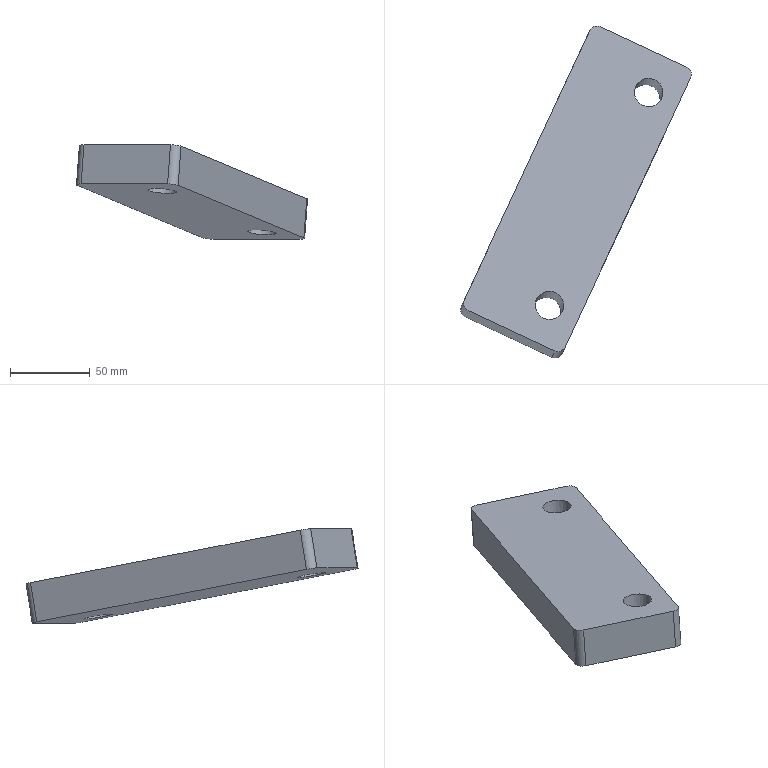Part | NX | features MAIN_BODY 2 | 1 solid | 12 faces | box 145.264 x 208.749 x 59.35 mm | volume 336740 mm3 | plane 6 | cylinder 6 | commonest cylinder face diameters 10 x4 18 x2
STEP:
#1=CARTESIAN_POINT('',(608.13,416.814,55.362));
#2=VERTEX_POINT('',#1);
#3=CARTESIAN_POINT('',(662.509,391.456,55.362));
#4=VERTEX_POINT('',#3);
#5=CARTESIAN_POINT('',(603.599,418.927,55.362));
#6=DIRECTION('',(0.9063,-0.4226,0.000000004));
#7=VECTOR('',#6,1000.);
#8=LINE('',#5,#7);
#9=EDGE_CURVE('',#2,#4,#8,.T.);
#10=ORIENTED_EDGE('',*,*,#9,.T.);
#11=CARTESIAN_POINT('',(664.343,395.391,79.982));
#12=VERTEX_POINT('',#11);
#13=CARTESIAN_POINT('',(664.343,395.391,79.982));
#14=DIRECTION('',(-0.07339,-0.1574,-0.9848));
#15=VECTOR('',#14,1000.);
#16=LINE('',#13,#15);
#17=EDGE_CURVE('',#12,#4,#16,.T.);
#18=ORIENTED_EDGE('',*,*,#17,.F.);
#19=CARTESIAN_POINT('',(609.965,420.748,79.982));
#20=VERTEX_POINT('',#19);
#21=CARTESIAN_POINT('',(605.433,422.861,79.982));
#22=DIRECTION('',(0.9063,-0.4226,0.000000004));
#23=VECTOR('',#22,1000.);
#24=LINE('',#21,#23);
#25=EDGE_CURVE('',#20,#12,#24,.T.);
#26=ORIENTED_EDGE('',*,*,#25,.F.);
#27=CARTESIAN_POINT('',(609.965,420.748,79.982));
#28=DIRECTION('',(-0.07339,-0.1574,-0.9848));
#29=VECTOR('',#28,1000.);
#30=LINE('',#27,#29);
#31=EDGE_CURVE('',#2,#20,#30,.F.);
#32=ORIENTED_EDGE('',*,*,#31,.F.);
#33=EDGE_LOOP('',(#10,#18,#26,#32));
#34=FACE_BOUND('',#33,.T.);
#35=CARTESIAN_POINT('',(605.433,422.861,79.982));
#36=DIRECTION('',(-0.4162,-0.8925,0.1736));
#37=DIRECTION('',(-0.9063,0.4226,-0.000000004));
#38=AXIS2_PLACEMENT_3D('',#35,#36,#37);
#39=PLANE('',#38);
#40=ADVANCED_FACE('',(#34),#39,.T.);
#41=CARTESIAN_POINT('',(670.956,397.741,79.114));
#42=VERTEX_POINT('',#41);
#43=CARTESIAN_POINT('',(750.033,567.323,46.121));
#44=VERTEX_POINT('',#43);
#45=CARTESIAN_POINT('',(668.875,393.278,79.982));
#46=DIRECTION('',(0.4162,0.8925,-0.1736));
#47=VECTOR('',#46,1000.);
#48=LINE('',#45,#47);
#49=EDGE_CURVE('',#42,#44,#48,.T.);
#50=ORIENTED_EDGE('',*,*,#49,.F.);
#51=CARTESIAN_POINT('',(669.121,393.806,54.494));
#52=VERTEX_POINT('',#51);
#53=CARTESIAN_POINT('',(670.956,397.741,79.114));
#54=DIRECTION('',(-0.07339,-0.1574,-0.9848));
#55=VECTOR('',#54,1000.);
#56=LINE('',#53,#55);
#57=EDGE_CURVE('',#52,#42,#56,.F.);
#58=ORIENTED_EDGE('',*,*,#57,.F.);
#59=CARTESIAN_POINT('',(748.199,563.388,21.501));
#60=VERTEX_POINT('',#59);
#61=CARTESIAN_POINT('',(667.04,389.343,55.362));
#62=DIRECTION('',(0.4162,0.8925,-0.1736));
#63=VECTOR('',#62,1000.);
#64=LINE('',#61,#63);
#65=EDGE_CURVE('',#52,#60,#64,.T.);
#66=ORIENTED_EDGE('',*,*,#65,.T.);
#67=CARTESIAN_POINT('',(750.033,567.323,46.121));
#68=DIRECTION('',(-0.07339,-0.1574,-0.9848));
#69=VECTOR('',#68,1000.);
#70=LINE('',#67,#69);
#71=EDGE_CURVE('',#44,#60,#70,.T.);
#72=ORIENTED_EDGE('',*,*,#71,.F.);
#73=EDGE_LOOP('',(#50,#58,#66,#72));
#74=FACE_BOUND('',#73,.T.);
#75=CARTESIAN_POINT('',(668.875,393.278,79.982));
#76=DIRECTION('',(0.9063,-0.4226,0.000000004));
#77=DIRECTION('',(-0.4162,-0.8925,0.1736));
#78=AXIS2_PLACEMENT_3D('',#75,#76,#77);
#79=PLANE('',#78);
#80=ADVANCED_FACE('',(#74),#79,.T.);
#81=CARTESIAN_POINT('',(747.583,573.899,45.252));
#82=VERTEX_POINT('',#81);
#83=CARTESIAN_POINT('',(693.204,599.256,45.252));
#84=VERTEX_POINT('',#83);
#85=CARTESIAN_POINT('',(752.114,571.786,45.252));
#86=DIRECTION('',(-0.9063,0.4226,-0.000000004));
#87=VECTOR('',#86,1000.);
#88=LINE('',#85,#87);
#89=EDGE_CURVE('',#82,#84,#88,.T.);
#90=ORIENTED_EDGE('',*,*,#89,.F.);
#91=CARTESIAN_POINT('',(745.748,569.964,20.632));
#92=VERTEX_POINT('',#91);
#93=CARTESIAN_POINT('',(747.583,573.899,45.252));
#94=DIRECTION('',(-0.07339,-0.1574,-0.9848));
#95=VECTOR('',#94,1000.);
#96=LINE('',#93,#95);
#97=EDGE_CURVE('',#92,#82,#96,.F.);
#98=ORIENTED_EDGE('',*,*,#97,.F.);
#99=CARTESIAN_POINT('',(691.37,595.321,20.632));
#100=VERTEX_POINT('',#99);
#101=CARTESIAN_POINT('',(750.28,567.851,20.632));
#102=DIRECTION('',(-0.9063,0.4226,-0.000000004));
#103=VECTOR('',#102,1000.);
#104=LINE('',#101,#103);
#105=EDGE_CURVE('',#92,#100,#104,.T.);
#106=ORIENTED_EDGE('',*,*,#105,.T.);
#107=CARTESIAN_POINT('',(693.204,599.256,45.252));
#108=DIRECTION('',(-0.07339,-0.1574,-0.9848));
#109=VECTOR('',#108,1000.);
#110=LINE('',#107,#109);
#111=EDGE_CURVE('',#84,#100,#110,.T.);
#112=ORIENTED_EDGE('',*,*,#111,.F.);
#113=EDGE_LOOP('',(#90,#98,#106,#112));
#114=FACE_BOUND('',#113,.T.);
#115=CARTESIAN_POINT('',(752.114,571.786,45.252));
#116=DIRECTION('',(0.4162,0.8925,-0.1736));
#117=DIRECTION('',(0.07339,0.1574,0.9848));
#118=AXIS2_PLACEMENT_3D('',#115,#116,#117);
#119=PLANE('',#118);
#120=ADVANCED_FACE('',(#114),#119,.T.);
#121=CARTESIAN_POINT('',(684.757,592.972,21.501));
#122=VERTEX_POINT('',#121);
#123=CARTESIAN_POINT('',(605.68,423.389,54.494));
#124=VERTEX_POINT('',#123);
#125=CARTESIAN_POINT('',(686.838,597.434,20.632));
#126=DIRECTION('',(-0.4162,-0.8925,0.1736));
#127=VECTOR('',#126,1000.);
#128=LINE('',#125,#127);
#129=EDGE_CURVE('',#122,#124,#128,.T.);
#130=ORIENTED_EDGE('',*,*,#129,.T.);
#131=CARTESIAN_POINT('',(607.514,427.324,79.114));
#132=VERTEX_POINT('',#131);
#133=CARTESIAN_POINT('',(607.514,427.324,79.114));
#134=DIRECTION('',(-0.07339,-0.1574,-0.9848));
#135=VECTOR('',#134,1000.);
#136=LINE('',#133,#135);
#137=EDGE_CURVE('',#132,#124,#136,.T.);
#138=ORIENTED_EDGE('',*,*,#137,.F.);
#139=CARTESIAN_POINT('',(686.592,596.906,46.121));
#140=VERTEX_POINT('',#139);
#141=CARTESIAN_POINT('',(688.673,601.369,45.252));
#142=DIRECTION('',(-0.4162,-0.8925,0.1736));
#143=VECTOR('',#142,1000.);
#144=LINE('',#141,#143);
#145=EDGE_CURVE('',#140,#132,#144,.T.);
#146=ORIENTED_EDGE('',*,*,#145,.F.);
#147=CARTESIAN_POINT('',(686.592,596.906,46.121));
#148=DIRECTION('',(-0.07339,-0.1574,-0.9848));
#149=VECTOR('',#148,1000.);
#150=LINE('',#147,#149);
#151=EDGE_CURVE('',#122,#140,#150,.F.);
#152=ORIENTED_EDGE('',*,*,#151,.F.);
#153=EDGE_LOOP('',(#130,#138,#146,#152));
#154=FACE_BOUND('',#153,.T.);
#155=CARTESIAN_POINT('',(688.673,601.369,45.252));
#156=DIRECTION('',(-0.9063,0.4226,-0.000000004));
#157=DIRECTION('',(0.07339,0.1574,0.9848));
#158=AXIS2_PLACEMENT_3D('',#155,#156,#157);
#159=PLANE('',#158);
#160=ADVANCED_FACE('',(#154),#159,.T.);
#161=CARTESIAN_POINT('',(727.329,565.957,48.031));
#162=VERTEX_POINT('',#161);
#163=CARTESIAN_POINT('',(723.583,557.925,49.594));
#164=DIRECTION('',(0.07339,0.1574,0.9848));
#165=DIRECTION('',(0.4162,0.8925,-0.1736));
#166=AXIS2_PLACEMENT_3D('',#163,#164,#165);
#167=CIRCLE('',#166,9.);
#168=EDGE_CURVE('',#162,#162,#167,.T.);
#169=ORIENTED_EDGE('',*,*,#168,.F.);
#170=EDGE_LOOP('',(#169));
#171=FACE_BOUND('',#170,.T.);
#172=CARTESIAN_POINT('',(664.899,432.077,74.078));
#173=VERTEX_POINT('',#172);
#174=CARTESIAN_POINT('',(661.154,424.044,75.641));
#175=DIRECTION('',(0.07339,0.1574,0.9848));
#176=DIRECTION('',(0.4162,0.8925,-0.1736));
#177=AXIS2_PLACEMENT_3D('',#174,#175,#176);
#178=CIRCLE('',#177,9.);
#179=EDGE_CURVE('',#173,#173,#178,.T.);
#180=ORIENTED_EDGE('',*,*,#179,.F.);
#181=EDGE_LOOP('',(#180));
#182=FACE_BOUND('',#181,.T.);
#183=ORIENTED_EDGE('',*,*,#145,.T.);
#184=CARTESIAN_POINT('',(612.046,425.211,79.114));
#185=DIRECTION('',(0.07339,0.1574,0.9848));
#186=DIRECTION('',(0.4162,0.8925,-0.1736));
#187=AXIS2_PLACEMENT_3D('',#184,#185,#186);
#188=CIRCLE('',#187,5.);
#189=EDGE_CURVE('',#20,#132,#188,.F.);
#190=ORIENTED_EDGE('',*,*,#189,.F.);
#191=ORIENTED_EDGE('',*,*,#25,.T.);
#192=CARTESIAN_POINT('',(666.424,399.854,79.114));
#193=DIRECTION('',(0.07339,0.1574,0.9848));
#194=DIRECTION('',(0.4162,0.8925,-0.1736));
#195=AXIS2_PLACEMENT_3D('',#192,#193,#194);
#196=CIRCLE('',#195,5.);
#197=EDGE_CURVE('',#42,#12,#196,.F.);
#198=ORIENTED_EDGE('',*,*,#197,.F.);
#199=ORIENTED_EDGE('',*,*,#49,.T.);
#200=CARTESIAN_POINT('',(745.502,569.436,46.121));
#201=DIRECTION('',(0.07339,0.1574,0.9848));
#202=DIRECTION('',(0.4162,0.8925,-0.1736));
#203=AXIS2_PLACEMENT_3D('',#200,#201,#202);
#204=CIRCLE('',#203,5.);
#205=EDGE_CURVE('',#82,#44,#204,.F.);
#206=ORIENTED_EDGE('',*,*,#205,.F.);
#207=ORIENTED_EDGE('',*,*,#89,.T.);
#208=CARTESIAN_POINT('',(691.123,594.793,46.121));
#209=DIRECTION('',(0.07339,0.1574,0.9848));
#210=DIRECTION('',(0.4162,0.8925,-0.1736));
#211=AXIS2_PLACEMENT_3D('',#208,#209,#210);
#212=CIRCLE('',#211,5.);
#213=EDGE_CURVE('',#140,#84,#212,.F.);
#214=ORIENTED_EDGE('',*,*,#213,.F.);
#215=EDGE_LOOP('',(#183,#190,#191,#198,#199,#206,#207,#214));
#216=FACE_BOUND('',#215,.T.);
#217=CARTESIAN_POINT('',(668.875,393.278,79.982));
#218=DIRECTION('',(-0.07339,-0.1574,-0.9848));
#219=DIRECTION('',(0.4162,0.8925,-0.1736));
#220=AXIS2_PLACEMENT_3D('',#217,#218,#219);
#221=PLANE('',#220);
#222=ADVANCED_FACE('',(#171,#182,#216),#221,.F.);
#223=CARTESIAN_POINT('',(725.494,562.023,23.411));
#224=VERTEX_POINT('',#223);
#225=CARTESIAN_POINT('',(721.749,553.99,24.974));
#226=DIRECTION('',(0.07339,0.1574,0.9848));
#227=DIRECTION('',(0.4162,0.8925,-0.1736));
#228=AXIS2_PLACEMENT_3D('',#225,#226,#227);
#229=CIRCLE('',#228,9.);
#230=EDGE_CURVE('',#224,#224,#229,.T.);
#231=ORIENTED_EDGE('',*,*,#230,.T.);
#232=EDGE_LOOP('',(#231));
#233=FACE_BOUND('',#232,.T.);
#234=CARTESIAN_POINT('',(663.065,428.142,49.458));
#235=VERTEX_POINT('',#234);
#236=CARTESIAN_POINT('',(659.319,420.109,51.021));
#237=DIRECTION('',(0.07339,0.1574,0.9848));
#238=DIRECTION('',(0.4162,0.8925,-0.1736));
#239=AXIS2_PLACEMENT_3D('',#236,#237,#238);
#240=CIRCLE('',#239,9.);
#241=EDGE_CURVE('',#235,#235,#240,.T.);
#242=ORIENTED_EDGE('',*,*,#241,.T.);
#243=EDGE_LOOP('',(#242));
#244=FACE_BOUND('',#243,.T.);
#245=ORIENTED_EDGE('',*,*,#105,.F.);
#246=CARTESIAN_POINT('',(743.667,565.502,21.501));
#247=DIRECTION('',(0.07339,0.1574,0.9848));
#248=DIRECTION('',(0.4162,0.8925,-0.1736));
#249=AXIS2_PLACEMENT_3D('',#246,#247,#248);
#250=CIRCLE('',#249,5.);
#251=EDGE_CURVE('',#60,#92,#250,.T.);
#252=ORIENTED_EDGE('',*,*,#251,.F.);
#253=ORIENTED_EDGE('',*,*,#65,.F.);
#254=CARTESIAN_POINT('',(664.59,395.919,54.494));
#255=DIRECTION('',(0.07339,0.1574,0.9848));
#256=DIRECTION('',(0.4162,0.8925,-0.1736));
#257=AXIS2_PLACEMENT_3D('',#254,#255,#256);
#258=CIRCLE('',#257,5.);
#259=EDGE_CURVE('',#4,#52,#258,.T.);
#260=ORIENTED_EDGE('',*,*,#259,.F.);
#261=ORIENTED_EDGE('',*,*,#9,.F.);
#262=CARTESIAN_POINT('',(610.211,421.276,54.494));
#263=DIRECTION('',(0.07339,0.1574,0.9848));
#264=DIRECTION('',(0.4162,0.8925,-0.1736));
#265=AXIS2_PLACEMENT_3D('',#262,#263,#264);
#266=CIRCLE('',#265,5.);
#267=EDGE_CURVE('',#124,#2,#266,.T.);
#268=ORIENTED_EDGE('',*,*,#267,.F.);
#269=ORIENTED_EDGE('',*,*,#129,.F.);
#270=CARTESIAN_POINT('',(689.289,590.859,21.501));
#271=DIRECTION('',(0.07339,0.1574,0.9848));
#272=DIRECTION('',(0.4162,0.8925,-0.1736));
#273=AXIS2_PLACEMENT_3D('',#270,#271,#272);
#274=CIRCLE('',#273,5.);
#275=EDGE_CURVE('',#100,#122,#274,.T.);
#276=ORIENTED_EDGE('',*,*,#275,.F.);
#277=EDGE_LOOP('',(#245,#252,#253,#260,#261,#268,#269,#276));
#278=FACE_BOUND('',#277,.T.);
#279=CARTESIAN_POINT('',(667.04,389.343,55.362));
#280=DIRECTION('',(-0.07339,-0.1574,-0.9848));
#281=DIRECTION('',(0.4162,0.8925,-0.1736));
#282=AXIS2_PLACEMENT_3D('',#279,#280,#281);
#283=PLANE('',#282);
#284=ADVANCED_FACE('',(#233,#244,#278),#283,.T.);
#285=ORIENTED_EDGE('',*,*,#241,.F.);
#286=EDGE_LOOP('',(#285));
#287=FACE_BOUND('',#286,.T.);
#288=ORIENTED_EDGE('',*,*,#179,.T.);
#289=EDGE_LOOP('',(#288));
#290=FACE_BOUND('',#289,.T.);
#291=CARTESIAN_POINT('',(661.154,424.044,75.641));
#292=DIRECTION('',(-0.07339,-0.1574,-0.9848));
#293=DIRECTION('',(0.4162,0.8925,-0.1736));
#294=AXIS2_PLACEMENT_3D('',#291,#292,#293);
#295=CYLINDRICAL_SURFACE('',#294,9.);
#296=ADVANCED_FACE('',(#287,#290),#295,.F.);
#297=ORIENTED_EDGE('',*,*,#230,.F.);
#298=EDGE_LOOP('',(#297));
#299=FACE_BOUND('',#298,.T.);
#300=ORIENTED_EDGE('',*,*,#168,.T.);
#301=EDGE_LOOP('',(#300));
#302=FACE_BOUND('',#301,.T.);
#303=CARTESIAN_POINT('',(723.583,557.925,49.594));
#304=DIRECTION('',(-0.07339,-0.1574,-0.9848));
#305=DIRECTION('',(0.4162,0.8925,-0.1736));
#306=AXIS2_PLACEMENT_3D('',#303,#304,#305);
#307=CYLINDRICAL_SURFACE('',#306,9.);
#308=ADVANCED_FACE('',(#299,#302),#307,.F.);
#309=ORIENTED_EDGE('',*,*,#213,.T.);
#310=ORIENTED_EDGE('',*,*,#111,.T.);
#311=ORIENTED_EDGE('',*,*,#275,.T.);
#312=ORIENTED_EDGE('',*,*,#151,.T.);
#313=EDGE_LOOP('',(#309,#310,#311,#312));
#314=FACE_BOUND('',#313,.T.);
#315=CARTESIAN_POINT('',(691.123,594.793,46.121));
#316=DIRECTION('',(-0.07339,-0.1574,-0.9848));
#317=DIRECTION('',(0.4162,0.8925,-0.1736));
#318=AXIS2_PLACEMENT_3D('',#315,#316,#317);
#319=CYLINDRICAL_SURFACE('',#318,5.);
#320=ADVANCED_FACE('',(#314),#319,.T.);
#321=ORIENTED_EDGE('',*,*,#205,.T.);
#322=ORIENTED_EDGE('',*,*,#71,.T.);
#323=ORIENTED_EDGE('',*,*,#251,.T.);
#324=ORIENTED_EDGE('',*,*,#97,.T.);
#325=EDGE_LOOP('',(#321,#322,#323,#324));
#326=FACE_BOUND('',#325,.T.);
#327=CARTESIAN_POINT('',(745.502,569.436,46.121));
#328=DIRECTION('',(-0.07339,-0.1574,-0.9848));
#329=DIRECTION('',(0.4162,0.8925,-0.1736));
#330=AXIS2_PLACEMENT_3D('',#327,#328,#329);
#331=CYLINDRICAL_SURFACE('',#330,5.);
#332=ADVANCED_FACE('',(#326),#331,.T.);
#333=ORIENTED_EDGE('',*,*,#189,.T.);
#334=ORIENTED_EDGE('',*,*,#137,.T.);
#335=ORIENTED_EDGE('',*,*,#267,.T.);
#336=ORIENTED_EDGE('',*,*,#31,.T.);
#337=EDGE_LOOP('',(#333,#334,#335,#336));
#338=FACE_BOUND('',#337,.T.);
#339=CARTESIAN_POINT('',(612.046,425.211,79.114));
#340=DIRECTION('',(-0.07339,-0.1574,-0.9848));
#341=DIRECTION('',(0.4162,0.8925,-0.1736));
#342=AXIS2_PLACEMENT_3D('',#339,#340,#341);
#343=CYLINDRICAL_SURFACE('',#342,5.);
#344=ADVANCED_FACE('',(#338),#343,.T.);
#345=ORIENTED_EDGE('',*,*,#197,.T.);
#346=ORIENTED_EDGE('',*,*,#17,.T.);
#347=ORIENTED_EDGE('',*,*,#259,.T.);
#348=ORIENTED_EDGE('',*,*,#57,.T.);
#349=EDGE_LOOP('',(#345,#346,#347,#348));
#350=FACE_BOUND('',#349,.T.);
#351=CARTESIAN_POINT('',(666.424,399.854,79.114));
#352=DIRECTION('',(-0.07339,-0.1574,-0.9848));
#353=DIRECTION('',(0.4162,0.8925,-0.1736));
#354=AXIS2_PLACEMENT_3D('',#351,#352,#353);
#355=CYLINDRICAL_SURFACE('',#354,5.);
#356=ADVANCED_FACE('',(#350),#355,.T.);
#357=CLOSED_SHELL('',(#40,#80,#120,#160,#222,#284,#296,#308,#320,#332,#344,#356));
#358=MANIFOLD_SOLID_BREP('',#357);
#359=(LENGTH_UNIT()NAMED_UNIT(*)SI_UNIT(.MILLI.,.METRE.));
#360=UNCERTAINTY_MEASURE_WITH_UNIT(LENGTH_MEASURE(0.00001),#359,'','');
#361=(NAMED_UNIT(*)PLANE_ANGLE_UNIT()SI_UNIT($,.RADIAN.));
#362=(NAMED_UNIT(*)SI_UNIT($,.STERADIAN.)SOLID_ANGLE_UNIT());
#363=(GEOMETRIC_REPRESENTATION_CONTEXT(3)GLOBAL_UNCERTAINTY_ASSIGNED_CONTEXT((#360))GLOBAL_UNIT_ASSIGNED_CONTEXT((#359,#361,#362))REPRESENTATION_CONTEXT('',''));
#364=ADVANCED_BREP_SHAPE_REPRESENTATION('',(#358),#363);